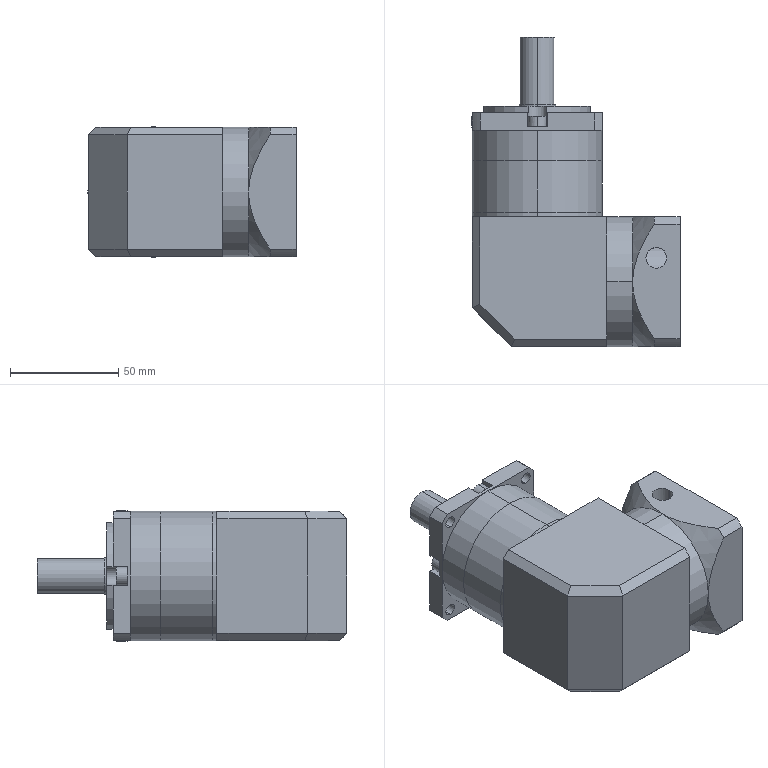Part | SolidWorks | features BaseBody 3 | 3 solids | 292 faces | box 96.25 x 143 x 60.5 mm | volume 444085 mm3 | plane 165 | cylinder 113 | cone 14 | commonest cylinder face diameters 9 x16 4.2 x12 17 x11 50 x9 5.5 x8 8.5 x8